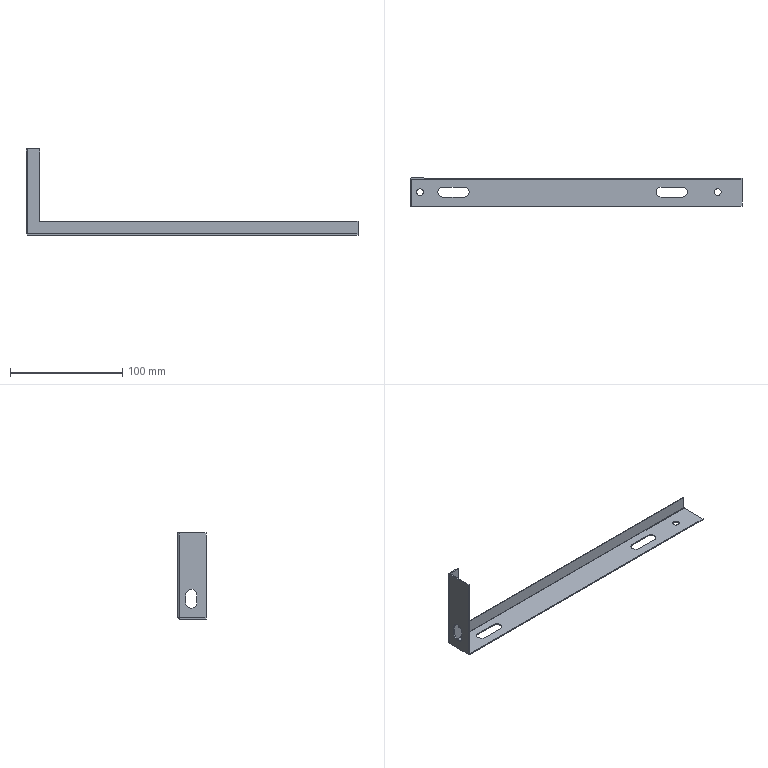Part | SolidWorks | features Cut 2, EdgeFlange 2, FlatPattern 1, ICE 1, LPattern 1, SMBaseFlange 1, SheetMetal 1 | 1 solid | 40 faces | box 296 x 25 x 76.7 mm | volume 12498 mm3 | plane 26 | cylinder 14 | commonest cylinder face diameters 6 x4 9 x4 0.4 x2 2.4 x2 10 x2
STEP:
#1=CARTESIAN_POINT('',(125.7,-15.5,-0.2));
#2=VERTEX_POINT('',#1);
#3=CARTESIAN_POINT('',(125.7,-9.5,-0.2));
#4=VERTEX_POINT('',#3);
#5=CARTESIAN_POINT('',(125.7,-12.5,-0.2));
#6=DIRECTION('',(0.,0.,-1.));
#7=DIRECTION('',(0.,1.,0.));
#8=AXIS2_PLACEMENT_3D('',#5,#6,#7);
#9=CIRCLE('',#8,3.);
#10=EDGE_CURVE('',#2,#4,#9,.T.);
#11=ORIENTED_EDGE('',*,*,#10,.F.);
#12=CARTESIAN_POINT('',(125.7,-15.5,-1.2));
#13=VERTEX_POINT('',#12);
#14=CARTESIAN_POINT('',(125.7,-15.5,8.8));
#15=DIRECTION('',(0.,0.,-1.));
#16=VECTOR('',#15,1000.);
#17=LINE('',#14,#16);
#18=EDGE_CURVE('',#2,#13,#17,.T.);
#19=ORIENTED_EDGE('',*,*,#18,.T.);
#20=CARTESIAN_POINT('',(125.7,-9.5,-1.2));
#21=VERTEX_POINT('',#20);
#22=CARTESIAN_POINT('',(125.7,-12.5,-1.2));
#23=DIRECTION('',(0.,0.,-1.));
#24=DIRECTION('',(0.,1.,0.));
#25=AXIS2_PLACEMENT_3D('',#22,#23,#24);
#26=CIRCLE('',#25,3.);
#27=EDGE_CURVE('',#13,#21,#26,.T.);
#28=ORIENTED_EDGE('',*,*,#27,.T.);
#29=CARTESIAN_POINT('',(125.7,-9.5,8.8));
#30=DIRECTION('',(0.,0.,-1.));
#31=VECTOR('',#30,1000.);
#32=LINE('',#29,#31);
#33=EDGE_CURVE('',#4,#21,#32,.T.);
#34=ORIENTED_EDGE('',*,*,#33,.F.);
#35=EDGE_LOOP('',(#11,#19,#28,#34));
#36=FACE_OUTER_BOUND('',#35,.T.);
#37=CARTESIAN_POINT('',(125.7,-12.5,8.8));
#38=DIRECTION('',(0.,0.,-1.));
#39=DIRECTION('',(0.,1.,0.));
#40=AXIS2_PLACEMENT_3D('',#37,#38,#39);
#41=CYLINDRICAL_SURFACE('',#40,3.);
#42=ADVANCED_FACE('',(#36),#41,.F.);
#43=CARTESIAN_POINT('',(-139.8,-15.5,-0.2));
#44=VERTEX_POINT('',#43);
#45=CARTESIAN_POINT('',(-139.8,-9.5,-0.2));
#46=VERTEX_POINT('',#45);
#47=CARTESIAN_POINT('',(-139.8,-12.5,-0.2));
#48=DIRECTION('',(0.,0.,-1.));
#49=DIRECTION('',(0.,1.,0.));
#50=AXIS2_PLACEMENT_3D('',#47,#48,#49);
#51=CIRCLE('',#50,3.);
#52=EDGE_CURVE('',#44,#46,#51,.T.);
#53=ORIENTED_EDGE('',*,*,#52,.F.);
#54=CARTESIAN_POINT('',(-139.8,-15.5,-1.2));
#55=VERTEX_POINT('',#54);
#56=CARTESIAN_POINT('',(-139.8,-15.5,8.8));
#57=DIRECTION('',(0.,0.,-1.));
#58=VECTOR('',#57,1000.);
#59=LINE('',#56,#58);
#60=EDGE_CURVE('',#44,#55,#59,.T.);
#61=ORIENTED_EDGE('',*,*,#60,.T.);
#62=CARTESIAN_POINT('',(-139.8,-9.5,-1.2));
#63=VERTEX_POINT('',#62);
#64=CARTESIAN_POINT('',(-139.8,-12.5,-1.2));
#65=DIRECTION('',(0.,0.,-1.));
#66=DIRECTION('',(0.,1.,0.));
#67=AXIS2_PLACEMENT_3D('',#64,#65,#66);
#68=CIRCLE('',#67,3.);
#69=EDGE_CURVE('',#55,#63,#68,.T.);
#70=ORIENTED_EDGE('',*,*,#69,.T.);
#71=CARTESIAN_POINT('',(-139.8,-9.5,8.8));
#72=DIRECTION('',(0.,0.,-1.));
#73=VECTOR('',#72,1000.);
#74=LINE('',#71,#73);
#75=EDGE_CURVE('',#46,#63,#74,.T.);
#76=ORIENTED_EDGE('',*,*,#75,.F.);
#77=EDGE_LOOP('',(#53,#61,#70,#76));
#78=FACE_OUTER_BOUND('',#77,.T.);
#79=CARTESIAN_POINT('',(-139.8,-12.5,8.8));
#80=DIRECTION('',(0.,0.,-1.));
#81=DIRECTION('',(0.,1.,0.));
#82=AXIS2_PLACEMENT_3D('',#79,#80,#81);
#83=CYLINDRICAL_SURFACE('',#82,3.);
#84=ADVANCED_FACE('',(#78),#83,.F.);
#85=CARTESIAN_POINT('',(147.4,-1.,11.));
#86=VERTEX_POINT('',#85);
#87=CARTESIAN_POINT('',(-136.4,-1.,11.));
#88=VERTEX_POINT('',#87);
#89=CARTESIAN_POINT('',(-147.4,-1.,11.));
#90=DIRECTION('',(-1.,0.,0.));
#91=VECTOR('',#90,1000.);
#92=LINE('',#89,#91);
#93=EDGE_CURVE('',#86,#88,#92,.T.);
#94=ORIENTED_EDGE('',*,*,#93,.T.);
#95=CARTESIAN_POINT('',(-136.4,-1.,75.5));
#96=VERTEX_POINT('',#95);
#97=CARTESIAN_POINT('',(-136.4,-1.,75.5));
#98=DIRECTION('',(0.,0.,1.));
#99=VECTOR('',#98,1000.);
#100=LINE('',#97,#99);
#101=EDGE_CURVE('',#88,#96,#100,.T.);
#102=ORIENTED_EDGE('',*,*,#101,.T.);
#103=CARTESIAN_POINT('',(-147.4,-1.,75.5));
#104=VERTEX_POINT('',#103);
#105=CARTESIAN_POINT('',(-147.4,-1.,75.5));
#106=DIRECTION('',(1.,0.,0.));
#107=VECTOR('',#106,1000.);
#108=LINE('',#105,#107);
#109=EDGE_CURVE('',#104,#96,#108,.T.);
#110=ORIENTED_EDGE('',*,*,#109,.F.);
#111=CARTESIAN_POINT('',(-147.4,-1.,0.));
#112=VERTEX_POINT('',#111);
#113=CARTESIAN_POINT('',(-147.4,-1.,75.5));
#114=DIRECTION('',(0.,0.,-1.));
#115=VECTOR('',#114,1000.);
#116=LINE('',#113,#115);
#117=EDGE_CURVE('',#104,#112,#116,.T.);
#118=ORIENTED_EDGE('',*,*,#117,.T.);
#119=CARTESIAN_POINT('',(147.4,-1.,0.));
#120=VERTEX_POINT('',#119);
#121=CARTESIAN_POINT('',(-147.4,-1.,0.));
#122=DIRECTION('',(1.,0.,0.));
#123=VECTOR('',#122,1000.);
#124=LINE('',#121,#123);
#125=EDGE_CURVE('',#112,#120,#124,.T.);
#126=ORIENTED_EDGE('',*,*,#125,.T.);
#127=CARTESIAN_POINT('',(147.4,-1.,75.5));
#128=DIRECTION('',(0.,0.,-1.));
#129=VECTOR('',#128,1000.);
#130=LINE('',#127,#129);
#131=EDGE_CURVE('',#86,#120,#130,.T.);
#132=ORIENTED_EDGE('',*,*,#131,.F.);
#133=EDGE_LOOP('',(#94,#102,#110,#118,#126,#132));
#134=FACE_OUTER_BOUND('',#133,.T.);
#135=CARTESIAN_POINT('',(-147.4,-1.,75.5));
#136=DIRECTION('',(0.,1.,0.));
#137=DIRECTION('',(-1.,0.,0.));
#138=AXIS2_PLACEMENT_3D('',#135,#136,#137);
#139=PLANE('',#138);
#140=ADVANCED_FACE('',(#134),#139,.F.);
#141=CARTESIAN_POINT('',(147.4,0.,11.));
#142=VERTEX_POINT('',#141);
#143=CARTESIAN_POINT('',(147.4,-10.,11.));
#144=DIRECTION('',(0.,1.,0.));
#145=VECTOR('',#144,1000.);
#146=LINE('',#143,#145);
#147=EDGE_CURVE('',#86,#142,#146,.T.);
#148=ORIENTED_EDGE('',*,*,#147,.F.);
#149=ORIENTED_EDGE('',*,*,#131,.T.);
#150=CARTESIAN_POINT('',(147.4,0.,0.));
#151=VERTEX_POINT('',#150);
#152=CARTESIAN_POINT('',(147.4,0.,0.));
#153=DIRECTION('',(0.,-1.,0.));
#154=VECTOR('',#153,1000.);
#155=LINE('',#152,#154);
#156=EDGE_CURVE('',#151,#120,#155,.T.);
#157=ORIENTED_EDGE('',*,*,#156,.F.);
#158=CARTESIAN_POINT('',(147.4,0.,75.5));
#159=DIRECTION('',(0.,0.,-1.));
#160=VECTOR('',#159,1000.);
#161=LINE('',#158,#160);
#162=EDGE_CURVE('',#142,#151,#161,.T.);
#163=ORIENTED_EDGE('',*,*,#162,.F.);
#164=EDGE_LOOP('',(#148,#149,#157,#163));
#165=FACE_OUTER_BOUND('',#164,.T.);
#166=CARTESIAN_POINT('',(147.4,0.,75.5));
#167=DIRECTION('',(1.,0.,0.));
#168=DIRECTION('',(0.,0.,-1.));
#169=AXIS2_PLACEMENT_3D('',#166,#167,#168);
#170=PLANE('',#169);
#171=ADVANCED_FACE('',(#165),#170,.T.);
#172=CARTESIAN_POINT('',(-136.4,0.,11.));
#173=VERTEX_POINT('',#172);
#174=CARTESIAN_POINT('',(-136.4,0.,75.5));
#175=VERTEX_POINT('',#174);
#176=CARTESIAN_POINT('',(-136.4,0.,75.5));
#177=DIRECTION('',(0.,0.,1.));
#178=VECTOR('',#177,1000.);
#179=LINE('',#176,#178);
#180=EDGE_CURVE('',#173,#175,#179,.T.);
#181=ORIENTED_EDGE('',*,*,#180,.F.);
#182=CARTESIAN_POINT('',(147.4,0.,11.));
#183=DIRECTION('',(-1.,0.,0.));
#184=VECTOR('',#183,1000.);
#185=LINE('',#182,#184);
#186=EDGE_CURVE('',#142,#173,#185,.T.);
#187=ORIENTED_EDGE('',*,*,#186,.F.);
#188=ORIENTED_EDGE('',*,*,#162,.T.);
#189=CARTESIAN_POINT('',(-147.4,0.,0.));
#190=VERTEX_POINT('',#189);
#191=CARTESIAN_POINT('',(-147.4,0.,0.));
#192=DIRECTION('',(1.,0.,0.));
#193=VECTOR('',#192,1000.);
#194=LINE('',#191,#193);
#195=EDGE_CURVE('',#190,#151,#194,.T.);
#196=ORIENTED_EDGE('',*,*,#195,.F.);
#197=CARTESIAN_POINT('',(-147.4,0.,75.5));
#198=VERTEX_POINT('',#197);
#199=CARTESIAN_POINT('',(-147.4,0.,75.5));
#200=DIRECTION('',(0.,0.,-1.));
#201=VECTOR('',#200,1000.);
#202=LINE('',#199,#201);
#203=EDGE_CURVE('',#198,#190,#202,.T.);
#204=ORIENTED_EDGE('',*,*,#203,.F.);
#205=CARTESIAN_POINT('',(-147.4,0.,75.5));
#206=DIRECTION('',(1.,0.,0.));
#207=VECTOR('',#206,1000.);
#208=LINE('',#205,#207);
#209=EDGE_CURVE('',#198,#175,#208,.T.);
#210=ORIENTED_EDGE('',*,*,#209,.T.);
#211=EDGE_LOOP('',(#181,#187,#188,#196,#204,#210));
#212=FACE_OUTER_BOUND('',#211,.T.);
#213=CARTESIAN_POINT('',(-147.4,0.,75.5));
#214=DIRECTION('',(0.,1.,0.));
#215=DIRECTION('',(-1.,0.,0.));
#216=AXIS2_PLACEMENT_3D('',#213,#214,#215);
#217=PLANE('',#216);
#218=ADVANCED_FACE('',(#212),#217,.T.);
#219=ORIENTED_EDGE('',*,*,#109,.T.);
#220=CARTESIAN_POINT('',(-136.4,0.,75.5));
#221=DIRECTION('',(0.,1.,0.));
#222=VECTOR('',#221,1000.);
#223=LINE('',#220,#222);
#224=EDGE_CURVE('',#96,#175,#223,.T.);
#225=ORIENTED_EDGE('',*,*,#224,.T.);
#226=ORIENTED_EDGE('',*,*,#209,.F.);
#227=CARTESIAN_POINT('',(-147.4,-1.,75.5));
#228=DIRECTION('',(0.,1.,0.));
#229=VECTOR('',#228,1000.);
#230=LINE('',#227,#229);
#231=EDGE_CURVE('',#104,#198,#230,.T.);
#232=ORIENTED_EDGE('',*,*,#231,.F.);
#233=EDGE_LOOP('',(#219,#225,#226,#232));
#234=FACE_OUTER_BOUND('',#233,.T.);
#235=CARTESIAN_POINT('',(0.,0.,75.5));
#236=DIRECTION('',(0.,0.,-1.));
#237=DIRECTION('',(-1.,0.,0.));
#238=AXIS2_PLACEMENT_3D('',#235,#236,#237);
#239=PLANE('',#238);
#240=ADVANCED_FACE('',(#234),#239,.F.);
#241=ORIENTED_EDGE('',*,*,#147,.T.);
#242=ORIENTED_EDGE('',*,*,#186,.T.);
#243=CARTESIAN_POINT('',(-136.4,-10.,11.));
#244=DIRECTION('',(0.,1.,0.));
#245=VECTOR('',#244,1000.);
#246=LINE('',#243,#245);
#247=EDGE_CURVE('',#88,#173,#246,.T.);
#248=ORIENTED_EDGE('',*,*,#247,.F.);
#249=ORIENTED_EDGE('',*,*,#93,.F.);
#250=EDGE_LOOP('',(#241,#242,#248,#249));
#251=FACE_OUTER_BOUND('',#250,.T.);
#252=CARTESIAN_POINT('',(147.4,-10.,11.));
#253=DIRECTION('',(0.,0.,-1.));
#254=DIRECTION('',(-1.,0.,0.));
#255=AXIS2_PLACEMENT_3D('',#252,#253,#254);
#256=PLANE('',#255);
#257=ADVANCED_FACE('',(#251),#256,.F.);
#258=ORIENTED_EDGE('',*,*,#247,.T.);
#259=ORIENTED_EDGE('',*,*,#180,.T.);
#260=ORIENTED_EDGE('',*,*,#224,.F.);
#261=ORIENTED_EDGE('',*,*,#101,.F.);
#262=EDGE_LOOP('',(#258,#259,#260,#261));
#263=FACE_OUTER_BOUND('',#262,.T.);
#264=CARTESIAN_POINT('',(-136.4,-10.,75.5));
#265=DIRECTION('',(-1.,0.,0.));
#266=DIRECTION('',(0.,0.,1.));
#267=AXIS2_PLACEMENT_3D('',#264,#265,#266);
#268=PLANE('',#267);
#269=ADVANCED_FACE('',(#263),#268,.F.);
#270=CARTESIAN_POINT('',(-147.4,-1.2,-0.2));
#271=VERTEX_POINT('',#270);
#272=CARTESIAN_POINT('',(-147.4,-1.2,-1.2));
#273=VERTEX_POINT('',#272);
#274=CARTESIAN_POINT('',(-147.4,-1.2,-1.2));
#275=DIRECTION('',(0.,0.,-1.));
#276=VECTOR('',#275,1000.);
#277=LINE('',#274,#276);
#278=EDGE_CURVE('',#271,#273,#277,.T.);
#279=ORIENTED_EDGE('',*,*,#278,.F.);
#280=CARTESIAN_POINT('',(-147.4,-1.2,0.));
#281=DIRECTION('',(-1.,0.,0.));
#282=DIRECTION('',(0.,1.,0.));
#283=AXIS2_PLACEMENT_3D('',#280,#281,#282);
#284=CIRCLE('',#283,0.2);
#285=EDGE_CURVE('',#112,#271,#284,.T.);
#286=ORIENTED_EDGE('',*,*,#285,.F.);
#287=CARTESIAN_POINT('',(-147.4,-1.,0.));
#288=DIRECTION('',(0.,1.,0.));
#289=VECTOR('',#288,1000.);
#290=LINE('',#287,#289);
#291=EDGE_CURVE('',#112,#190,#290,.T.);
#292=ORIENTED_EDGE('',*,*,#291,.T.);
#293=CARTESIAN_POINT('',(-147.4,-1.2,0.));
#294=DIRECTION('',(-1.,0.,0.));
#295=DIRECTION('',(0.,1.,0.));
#296=AXIS2_PLACEMENT_3D('',#293,#294,#295);
#297=CIRCLE('',#296,1.2);
#298=EDGE_CURVE('',#190,#273,#297,.T.);
#299=ORIENTED_EDGE('',*,*,#298,.T.);
#300=EDGE_LOOP('',(#279,#286,#292,#299));
#301=FACE_OUTER_BOUND('',#300,.T.);
#302=CARTESIAN_POINT('',(-147.4,-1.2,0.));
#303=DIRECTION('',(-1.,0.,0.));
#304=DIRECTION('',(0.,-1.,0.));
#305=AXIS2_PLACEMENT_3D('',#302,#303,#304);
#306=PLANE('',#305);
#307=ADVANCED_FACE('',(#301),#306,.T.);
#308=CARTESIAN_POINT('',(147.4,-1.2,-0.2));
#309=VERTEX_POINT('',#308);
#310=CARTESIAN_POINT('',(147.4,-1.2,0.));
#311=DIRECTION('',(1.,0.,0.));
#312=DIRECTION('',(0.,1.,0.));
#313=AXIS2_PLACEMENT_3D('',#310,#311,#312);
#314=CIRCLE('',#313,0.2);
#315=EDGE_CURVE('',#309,#120,#314,.T.);
#316=ORIENTED_EDGE('',*,*,#315,.F.);
#317=CARTESIAN_POINT('',(147.4,-1.2,-1.2));
#318=VERTEX_POINT('',#317);
#319=CARTESIAN_POINT('',(147.4,-1.2,-0.2));
#320=DIRECTION('',(0.,0.,-1.));
#321=VECTOR('',#320,1000.);
#322=LINE('',#319,#321);
#323=EDGE_CURVE('',#309,#318,#322,.T.);
#324=ORIENTED_EDGE('',*,*,#323,.T.);
#325=CARTESIAN_POINT('',(147.4,-1.2,0.));
#326=DIRECTION('',(1.,0.,0.));
#327=DIRECTION('',(0.,1.,0.));
#328=AXIS2_PLACEMENT_3D('',#325,#326,#327);
#329=CIRCLE('',#328,1.2);
#330=EDGE_CURVE('',#318,#151,#329,.T.);
#331=ORIENTED_EDGE('',*,*,#330,.T.);
#332=ORIENTED_EDGE('',*,*,#156,.T.);
#333=EDGE_LOOP('',(#316,#324,#331,#332));
#334=FACE_OUTER_BOUND('',#333,.T.);
#335=CARTESIAN_POINT('',(147.4,-1.2,0.));
#336=DIRECTION('',(-1.,0.,0.));
#337=DIRECTION('',(0.,-1.,0.));
#338=AXIS2_PLACEMENT_3D('',#335,#336,#337);
#339=PLANE('',#338);
#340=ADVANCED_FACE('',(#334),#339,.F.);
#341=ORIENTED_EDGE('',*,*,#195,.T.);
#342=ORIENTED_EDGE('',*,*,#330,.F.);
#343=CARTESIAN_POINT('',(0.,-1.2,-1.2));
#344=DIRECTION('',(1.,0.,0.));
#345=VECTOR('',#344,1000.);
#346=LINE('',#343,#345);
#347=EDGE_CURVE('',#273,#318,#346,.T.);
#348=ORIENTED_EDGE('',*,*,#347,.F.);
#349=ORIENTED_EDGE('',*,*,#298,.F.);
#350=EDGE_LOOP('',(#341,#342,#348,#349));
#351=FACE_OUTER_BOUND('',#350,.T.);
#352=CARTESIAN_POINT('',(147.4,-1.2,0.));
#353=DIRECTION('',(1.,0.,0.));
#354=DIRECTION('',(0.,0.,-1.));
#355=AXIS2_PLACEMENT_3D('',#352,#353,#354);
#356=CYLINDRICAL_SURFACE('',#355,1.2);
#357=ADVANCED_FACE('',(#351),#356,.T.);
#358=ORIENTED_EDGE('',*,*,#125,.F.);
#359=ORIENTED_EDGE('',*,*,#285,.T.);
#360=CARTESIAN_POINT('',(-147.4,-1.2,-0.2));
#361=DIRECTION('',(1.,0.,0.));
#362=VECTOR('',#361,1000.);
#363=LINE('',#360,#362);
#364=EDGE_CURVE('',#271,#309,#363,.T.);
#365=ORIENTED_EDGE('',*,*,#364,.T.);
#366=ORIENTED_EDGE('',*,*,#315,.T.);
#367=EDGE_LOOP('',(#358,#359,#365,#366));
#368=FACE_OUTER_BOUND('',#367,.T.);
#369=CARTESIAN_POINT('',(147.4,-1.2,0.));
#370=DIRECTION('',(1.,0.,0.));
#371=DIRECTION('',(0.,0.,-1.));
#372=AXIS2_PLACEMENT_3D('',#369,#370,#371);
#373=CYLINDRICAL_SURFACE('',#372,0.2);
#374=ADVANCED_FACE('',(#368),#373,.F.);
#375=CARTESIAN_POINT('',(147.4,-25.,-1.2));
#376=VERTEX_POINT('',#375);
#377=CARTESIAN_POINT('',(147.4,-1.,-1.2));
#378=DIRECTION('',(0.,1.,0.));
#379=VECTOR('',#378,1000.);
#380=LINE('',#377,#379);
#381=EDGE_CURVE('',#376,#318,#380,.T.);
#382=ORIENTED_EDGE('',*,*,#381,.T.);
#383=ORIENTED_EDGE('',*,*,#323,.F.);
#384=CARTESIAN_POINT('',(147.4,-25.,-0.2));
#385=VERTEX_POINT('',#384);
#386=CARTESIAN_POINT('',(147.4,0.,-0.2));
#387=DIRECTION('',(0.,1.,0.));
#388=VECTOR('',#387,1000.);
#389=LINE('',#386,#388);
#390=EDGE_CURVE('',#385,#309,#389,.T.);
#391=ORIENTED_EDGE('',*,*,#390,.F.);
#392=CARTESIAN_POINT('',(147.4,-25.,-1.2));
#393=DIRECTION('',(0.,0.,1.));
#394=VECTOR('',#393,1000.);
#395=LINE('',#392,#394);
#396=EDGE_CURVE('',#376,#385,#395,.T.);
#397=ORIENTED_EDGE('',*,*,#396,.F.);
#398=EDGE_LOOP('',(#382,#383,#391,#397));
#399=FACE_OUTER_BOUND('',#398,.T.);
#400=CARTESIAN_POINT('',(147.4,-1.,-1.2));
#401=DIRECTION('',(1.,0.,0.));
#402=DIRECTION('',(0.,0.,-1.));
#403=AXIS2_PLACEMENT_3D('',#400,#401,#402);
#404=PLANE('',#403);
#405=ADVANCED_FACE('',(#399),#404,.T.);
#406=CARTESIAN_POINT('',(-147.4,-25.,-0.2));
#407=VERTEX_POINT('',#406);
#408=CARTESIAN_POINT('',(-147.4,0.,-0.2));
#409=DIRECTION('',(0.,-1.,0.));
#410=VECTOR('',#409,1000.);
#411=LINE('',#408,#410);
#412=EDGE_CURVE('',#271,#407,#411,.T.);
#413=ORIENTED_EDGE('',*,*,#412,.F.);
#414=ORIENTED_EDGE('',*,*,#278,.T.);
#415=CARTESIAN_POINT('',(-147.4,-25.,-1.2));
#416=VERTEX_POINT('',#415);
#417=CARTESIAN_POINT('',(-147.4,-25.,-1.2));
#418=DIRECTION('',(0.,-1.,0.));
#419=VECTOR('',#418,1000.);
#420=LINE('',#417,#419);
#421=EDGE_CURVE('',#273,#416,#420,.T.);
#422=ORIENTED_EDGE('',*,*,#421,.T.);
#423=CARTESIAN_POINT('',(-147.4,-25.,-1.2));
#424=DIRECTION('',(0.,0.,1.));
#425=VECTOR('',#424,1000.);
#426=LINE('',#423,#425);
#427=EDGE_CURVE('',#416,#407,#426,.T.);
#428=ORIENTED_EDGE('',*,*,#427,.T.);
#429=EDGE_LOOP('',(#413,#414,#422,#428));
#430=FACE_OUTER_BOUND('',#429,.T.);
#431=CARTESIAN_POINT('',(-147.4,-25.,-1.2));
#432=DIRECTION('',(-1.,0.,0.));
#433=DIRECTION('',(0.,0.,1.));
#434=AXIS2_PLACEMENT_3D('',#431,#432,#433);
#435=PLANE('',#434);
#436=ADVANCED_FACE('',(#430),#435,.T.);
#437=CARTESIAN_POINT('',(125.7,-12.5,-1.2));
#438=DIRECTION('',(0.,0.,-1.));
#439=DIRECTION('',(0.,1.,0.));
#440=AXIS2_PLACEMENT_3D('',#437,#438,#439);
#441=CIRCLE('',#440,3.);
#442=EDGE_CURVE('',#21,#13,#441,.T.);
#443=ORIENTED_EDGE('',*,*,#442,.F.);
#444=ORIENTED_EDGE('',*,*,#27,.F.);
#445=EDGE_LOOP('',(#443,#444));
#446=FACE_BOUND('',#445,.T.);
#447=CARTESIAN_POINT('',(-139.8,-12.5,-1.2));
#448=DIRECTION('',(0.,0.,-1.));
#449=DIRECTION('',(0.,1.,0.));
#450=AXIS2_PLACEMENT_3D('',#447,#448,#449);
#451=CIRCLE('',#450,3.);
#452=EDGE_CURVE('',#63,#55,#451,.T.);
#453=ORIENTED_EDGE('',*,*,#452,.F.);
#454=ORIENTED_EDGE('',*,*,#69,.F.);
#455=EDGE_LOOP('',(#453,#454));
#456=FACE_BOUND('',#455,.T.);
#457=CARTESIAN_POINT('',(75.2,-17.,-1.2));
#458=VERTEX_POINT('',#457);
#459=CARTESIAN_POINT('',(75.2,-8.,-1.2));
#460=VERTEX_POINT('',#459);
#461=CARTESIAN_POINT('',(75.2,-12.5,-1.2));
#462=DIRECTION('',(0.,0.,-1.));
#463=DIRECTION('',(0.,1.,0.));
#464=AXIS2_PLACEMENT_3D('',#461,#462,#463);
#465=CIRCLE('',#464,4.5);
#466=EDGE_CURVE('',#458,#460,#465,.T.);
#467=ORIENTED_EDGE('',*,*,#466,.F.);
#468=CARTESIAN_POINT('',(94.2,-17.,-1.2));
#469=VERTEX_POINT('',#468);
#470=CARTESIAN_POINT('',(75.2,-17.,-1.2));
#471=DIRECTION('',(-1.,0.,0.));
#472=VECTOR('',#471,1000.);
#473=LINE('',#470,#472);
#474=EDGE_CURVE('',#469,#458,#473,.T.);
#475=ORIENTED_EDGE('',*,*,#474,.F.);
#476=CARTESIAN_POINT('',(94.2,-8.,-1.2));
#477=VERTEX_POINT('',#476);
#478=CARTESIAN_POINT('',(94.2,-12.5,-1.2));
#479=DIRECTION('',(0.,0.,-1.));
#480=DIRECTION('',(0.,1.,0.));
#481=AXIS2_PLACEMENT_3D('',#478,#479,#480);
#482=CIRCLE('',#481,4.5);
#483=EDGE_CURVE('',#477,#469,#482,.T.);
#484=ORIENTED_EDGE('',*,*,#483,.F.);
#485=CARTESIAN_POINT('',(75.2,-8.,-1.2));
#486=DIRECTION('',(1.,0.,0.));
#487=VECTOR('',#486,1000.);
#488=LINE('',#485,#487);
#489=EDGE_CURVE('',#460,#477,#488,.T.);
#490=ORIENTED_EDGE('',*,*,#489,.F.);
#491=EDGE_LOOP('',(#467,#475,#484,#490));
#492=FACE_BOUND('',#491,.T.);
#493=CARTESIAN_POINT('',(-119.3,-17.,-1.2));
#494=VERTEX_POINT('',#493);
#495=CARTESIAN_POINT('',(-119.3,-8.,-1.2));
#496=VERTEX_POINT('',#495);
#497=CARTESIAN_POINT('',(-119.3,-12.5,-1.2));
#498=DIRECTION('',(0.,0.,-1.));
#499=DIRECTION('',(0.,1.,0.));
#500=AXIS2_PLACEMENT_3D('',#497,#498,#499);
#501=CIRCLE('',#500,4.5);
#502=EDGE_CURVE('',#494,#496,#501,.T.);
#503=ORIENTED_EDGE('',*,*,#502,.F.);
#504=CARTESIAN_POINT('',(-100.3,-17.,-1.2));
#505=VERTEX_POINT('',#504);
#506=CARTESIAN_POINT('',(-119.3,-17.,-1.2));
#507=DIRECTION('',(-1.,0.,0.));
#508=VECTOR('',#507,1000.);
#509=LINE('',#506,#508);
#510=EDGE_CURVE('',#505,#494,#509,.T.);
#511=ORIENTED_EDGE('',*,*,#510,.F.);
#512=CARTESIAN_POINT('',(-100.3,-8.,-1.2));
#513=VERTEX_POINT('',#512);
#514=CARTESIAN_POINT('',(-100.3,-12.5,-1.2));
#515=DIRECTION('',(0.,0.,-1.));
#516=DIRECTION('',(0.,1.,0.));
#517=AXIS2_PLACEMENT_3D('',#514,#515,#516);
#518=CIRCLE('',#517,4.5);
#519=EDGE_CURVE('',#513,#505,#518,.T.);
#520=ORIENTED_EDGE('',*,*,#519,.F.);
#521=CARTESIAN_POINT('',(-119.3,-8.,-1.2));
#522=DIRECTION('',(1.,0.,0.));
#523=VECTOR('',#522,1000.);
#524=LINE('',#521,#523);
#525=EDGE_CURVE('',#496,#513,#524,.T.);
#526=ORIENTED_EDGE('',*,*,#525,.F.);
#527=EDGE_LOOP('',(#503,#511,#520,#526));
#528=FACE_BOUND('',#527,.T.);
#529=ORIENTED_EDGE('',*,*,#421,.F.);
#530=ORIENTED_EDGE('',*,*,#347,.T.);
#531=ORIENTED_EDGE('',*,*,#381,.F.);
#532=CARTESIAN_POINT('',(147.4,-25.,-1.2));
#533=DIRECTION('',(1.,0.,0.));
#534=VECTOR('',#533,1000.);
#535=LINE('',#532,#534);
#536=EDGE_CURVE('',#416,#376,#535,.T.);
#537=ORIENTED_EDGE('',*,*,#536,.F.);
#538=EDGE_LOOP('',(#529,#530,#531,#537));
#539=FACE_OUTER_BOUND('',#538,.T.);
#540=CARTESIAN_POINT('',(0.,0.,-1.2));
#541=DIRECTION('',(0.,0.,-1.));
#542=DIRECTION('',(0.,1.,0.));
#543=AXIS2_PLACEMENT_3D('',#540,#541,#542);
#544=PLANE('',#543);
#545=ADVANCED_FACE('',(#446,#456,#492,#528,#539),#544,.T.);
#546=CARTESIAN_POINT('',(125.7,-12.5,-0.2));
#547=DIRECTION('',(0.,0.,-1.));
#548=DIRECTION('',(0.,1.,0.));
#549=AXIS2_PLACEMENT_3D('',#546,#547,#548);
#550=CIRCLE('',#549,3.);
#551=EDGE_CURVE('',#4,#2,#550,.T.);
#552=ORIENTED_EDGE('',*,*,#551,.T.);
#553=ORIENTED_EDGE('',*,*,#10,.T.);
#554=EDGE_LOOP('',(#552,#553));
#555=FACE_BOUND('',#554,.T.);
#556=CARTESIAN_POINT('',(-139.8,-12.5,-0.2));
#557=DIRECTION('',(0.,0.,-1.));
#558=DIRECTION('',(0.,1.,0.));
#559=AXIS2_PLACEMENT_3D('',#556,#557,#558);
#560=CIRCLE('',#559,3.);
#561=EDGE_CURVE('',#46,#44,#560,.T.);
#562=ORIENTED_EDGE('',*,*,#561,.T.);
#563=ORIENTED_EDGE('',*,*,#52,.T.);
#564=EDGE_LOOP('',(#562,#563));
#565=FACE_BOUND('',#564,.T.);
#566=CARTESIAN_POINT('',(94.2,-17.,-0.2));
#567=VERTEX_POINT('',#566);
#568=CARTESIAN_POINT('',(75.2,-17.,-0.2));
#569=VERTEX_POINT('',#568);
#570=CARTESIAN_POINT('',(0.,-17.,-0.2));
#571=DIRECTION('',(-1.,0.,0.));
#572=VECTOR('',#571,1000.);
#573=LINE('',#570,#572);
#574=EDGE_CURVE('',#567,#569,#573,.T.);
#575=ORIENTED_EDGE('',*,*,#574,.T.);
#576=CARTESIAN_POINT('',(75.2,-8.,-0.2));
#577=VERTEX_POINT('',#576);
#578=CARTESIAN_POINT('',(75.2,-12.5,-0.2));
#579=DIRECTION('',(0.,0.,-1.));
#580=DIRECTION('',(0.,1.,0.));
#581=AXIS2_PLACEMENT_3D('',#578,#579,#580);
#582=CIRCLE('',#581,4.5);
#583=EDGE_CURVE('',#569,#577,#582,.T.);
#584=ORIENTED_EDGE('',*,*,#583,.T.);
#585=CARTESIAN_POINT('',(94.2,-8.,-0.2));
#586=VERTEX_POINT('',#585);
#587=CARTESIAN_POINT('',(0.,-8.,-0.2));
#588=DIRECTION('',(1.,0.,0.));
#589=VECTOR('',#588,1000.);
#590=LINE('',#587,#589);
#591=EDGE_CURVE('',#577,#586,#590,.T.);
#592=ORIENTED_EDGE('',*,*,#591,.T.);
#593=CARTESIAN_POINT('',(94.2,-12.5,-0.2));
#594=DIRECTION('',(0.,0.,-1.));
#595=DIRECTION('',(0.,1.,0.));
#596=AXIS2_PLACEMENT_3D('',#593,#594,#595);
#597=CIRCLE('',#596,4.5);
#598=EDGE_CURVE('',#586,#567,#597,.T.);
#599=ORIENTED_EDGE('',*,*,#598,.T.);
#600=EDGE_LOOP('',(#575,#584,#592,#599));
#601=FACE_BOUND('',#600,.T.);
#602=CARTESIAN_POINT('',(-100.3,-17.,-0.2));
#603=VERTEX_POINT('',#602);
#604=CARTESIAN_POINT('',(-119.3,-17.,-0.2));
#605=VERTEX_POINT('',#604);
#606=CARTESIAN_POINT('',(0.,-17.,-0.2));
#607=DIRECTION('',(-1.,0.,0.));
#608=VECTOR('',#607,1000.);
#609=LINE('',#606,#608);
#610=EDGE_CURVE('',#603,#605,#609,.T.);
#611=ORIENTED_EDGE('',*,*,#610,.T.);
#612=CARTESIAN_POINT('',(-119.3,-8.,-0.2));
#613=VERTEX_POINT('',#612);
#614=CARTESIAN_POINT('',(-119.3,-12.5,-0.2));
#615=DIRECTION('',(0.,0.,-1.));
#616=DIRECTION('',(0.,1.,0.));
#617=AXIS2_PLACEMENT_3D('',#614,#615,#616);
#618=CIRCLE('',#617,4.5);
#619=EDGE_CURVE('',#605,#613,#618,.T.);
#620=ORIENTED_EDGE('',*,*,#619,.T.);
#621=CARTESIAN_POINT('',(-100.3,-8.,-0.2));
#622=VERTEX_POINT('',#621);
#623=CARTESIAN_POINT('',(0.,-8.,-0.2));
#624=DIRECTION('',(1.,0.,0.));
#625=VECTOR('',#624,1000.);
#626=LINE('',#623,#625);
#627=EDGE_CURVE('',#613,#622,#626,.T.);
#628=ORIENTED_EDGE('',*,*,#627,.T.);
#629=CARTESIAN_POINT('',(-100.3,-12.5,-0.2));
#630=DIRECTION('',(0.,0.,-1.));
#631=DIRECTION('',(0.,1.,0.));
#632=AXIS2_PLACEMENT_3D('',#629,#630,#631);
#633=CIRCLE('',#632,4.5);
#634=EDGE_CURVE('',#622,#603,#633,.T.);
#635=ORIENTED_EDGE('',*,*,#634,.T.);
#636=EDGE_LOOP('',(#611,#620,#628,#635));
#637=FACE_BOUND('',#636,.T.);
#638=ORIENTED_EDGE('',*,*,#364,.F.);
#639=ORIENTED_EDGE('',*,*,#412,.T.);
#640=CARTESIAN_POINT('',(0.,-25.,-0.2));
#641=DIRECTION('',(1.,0.,0.));
#642=VECTOR('',#641,1000.);
#643=LINE('',#640,#642);
#644=EDGE_CURVE('',#407,#385,#643,.T.);
#645=ORIENTED_EDGE('',*,*,#644,.T.);
#646=ORIENTED_EDGE('',*,*,#390,.T.);
#647=EDGE_LOOP('',(#638,#639,#645,#646));
#648=FACE_OUTER_BOUND('',#647,.T.);
#649=CARTESIAN_POINT('',(0.,0.,-0.2));
#650=DIRECTION('',(0.,0.,-1.));
#651=DIRECTION('',(0.,1.,0.));
#652=AXIS2_PLACEMENT_3D('',#649,#650,#651);
#653=PLANE('',#652);
#654=ADVANCED_FACE('',(#555,#565,#601,#637,#648),#653,.F.);
#655=ORIENTED_EDGE('',*,*,#644,.F.);
#656=ORIENTED_EDGE('',*,*,#427,.F.);
#657=ORIENTED_EDGE('',*,*,#536,.T.);
#658=ORIENTED_EDGE('',*,*,#396,.T.);
#659=EDGE_LOOP('',(#655,#656,#657,#658));
#660=FACE_OUTER_BOUND('',#659,.T.);
#661=CARTESIAN_POINT('',(147.4,-25.,-1.2));
#662=DIRECTION('',(0.,-1.,0.));
#663=DIRECTION('',(0.,0.,-1.));
#664=AXIS2_PLACEMENT_3D('',#661,#662,#663);
#665=PLANE('',#664);
#666=ADVANCED_FACE('',(#660),#665,.T.);
#667=CARTESIAN_POINT('',(-147.6,-1.2,75.5));
#668=VERTEX_POINT('',#667);
#669=CARTESIAN_POINT('',(-148.6,-1.2,75.5));
#670=VERTEX_POINT('',#669);
#671=CARTESIAN_POINT('',(-148.6,-1.2,75.5));
#672=DIRECTION('',(-1.,0.,0.));
#673=VECTOR('',#672,1000.);
#674=LINE('',#671,#673);
#675=EDGE_CURVE('',#668,#670,#674,.T.);
#676=ORIENTED_EDGE('',*,*,#675,.F.);
#677=CARTESIAN_POINT('',(-147.4,-1.2,75.5));
#678=DIRECTION('',(0.,0.,1.));
#679=DIRECTION('',(-1.,0.,0.));
#680=AXIS2_PLACEMENT_3D('',#677,#678,#679);
#681=CIRCLE('',#680,0.2);
#682=EDGE_CURVE('',#104,#668,#681,.T.);
#683=ORIENTED_EDGE('',*,*,#682,.F.);
#684=ORIENTED_EDGE('',*,*,#231,.T.);
#685=CARTESIAN_POINT('',(-147.4,-1.2,75.5));
#686=DIRECTION('',(0.,0.,1.));
#687=DIRECTION('',(-1.,0.,0.));
#688=AXIS2_PLACEMENT_3D('',#685,#686,#687);
#689=CIRCLE('',#688,1.2);
#690=EDGE_CURVE('',#198,#670,#689,.T.);
#691=ORIENTED_EDGE('',*,*,#690,.T.);
#692=EDGE_LOOP('',(#676,#683,#684,#691));
#693=FACE_OUTER_BOUND('',#692,.T.);
#694=CARTESIAN_POINT('',(-147.4,-1.2,75.5));
#695=DIRECTION('',(0.,0.,1.));
#696=DIRECTION('',(1.,0.,0.));
#697=AXIS2_PLACEMENT_3D('',#694,#695,#696);
#698=PLANE('',#697);
#699=ADVANCED_FACE('',(#693),#698,.T.);
#700=CARTESIAN_POINT('',(-147.6,-1.2,0.));
#701=VERTEX_POINT('',#700);
#702=CARTESIAN_POINT('',(-147.4,-1.2,0.));
#703=DIRECTION('',(0.,0.,-1.));
#704=DIRECTION('',(-1.,0.,0.));
#705=AXIS2_PLACEMENT_3D('',#702,#703,#704);
#706=CIRCLE('',#705,0.2);
#707=EDGE_CURVE('',#701,#112,#706,.T.);
#708=ORIENTED_EDGE('',*,*,#707,.F.);
#709=CARTESIAN_POINT('',(-148.6,-1.2,0.));
#710=VERTEX_POINT('',#709);
#711=CARTESIAN_POINT('',(-147.6,-1.2,0.));
#712=DIRECTION('',(-1.,0.,0.));
#713=VECTOR('',#712,1000.);
#714=LINE('',#711,#713);
#715=EDGE_CURVE('',#701,#710,#714,.T.);
#716=ORIENTED_EDGE('',*,*,#715,.T.);
#717=CARTESIAN_POINT('',(-147.4,-1.2,0.));
#718=DIRECTION('',(0.,0.,-1.));
#719=DIRECTION('',(-1.,0.,0.));
#720=AXIS2_PLACEMENT_3D('',#717,#718,#719);
#721=CIRCLE('',#720,1.2);
#722=EDGE_CURVE('',#710,#190,#721,.T.);
#723=ORIENTED_EDGE('',*,*,#722,.T.);
#724=ORIENTED_EDGE('',*,*,#291,.F.);
#725=EDGE_LOOP('',(#708,#716,#723,#724));
#726=FACE_OUTER_BOUND('',#725,.T.);
#727=CARTESIAN_POINT('',(-147.4,-1.2,0.));
#728=DIRECTION('',(0.,0.,1.));
#729=DIRECTION('',(1.,0.,0.));
#730=AXIS2_PLACEMENT_3D('',#727,#728,#729);
#731=PLANE('',#730);
#732=ADVANCED_FACE('',(#726),#731,.F.);
#733=ORIENTED_EDGE('',*,*,#203,.T.);
#734=ORIENTED_EDGE('',*,*,#722,.F.);
#735=CARTESIAN_POINT('',(-148.6,-1.2,0.));
#736=DIRECTION('',(0.,0.,-1.));
#737=VECTOR('',#736,1000.);
#738=LINE('',#735,#737);
#739=EDGE_CURVE('',#670,#710,#738,.T.);
#740=ORIENTED_EDGE('',*,*,#739,.F.);
#741=ORIENTED_EDGE('',*,*,#690,.F.);
#742=EDGE_LOOP('',(#733,#734,#740,#741));
#743=FACE_OUTER_BOUND('',#742,.T.);
#744=CARTESIAN_POINT('',(-147.4,-1.2,0.));
#745=DIRECTION('',(0.,0.,-1.));
#746=DIRECTION('',(-1.,0.,0.));
#747=AXIS2_PLACEMENT_3D('',#744,#745,#746);
#748=CYLINDRICAL_SURFACE('',#747,1.2);
#749=ADVANCED_FACE('',(#743),#748,.T.);
#750=ORIENTED_EDGE('',*,*,#117,.F.);
#751=ORIENTED_EDGE('',*,*,#682,.T.);
#752=CARTESIAN_POINT('',(-147.6,-1.2,75.5));
#753=DIRECTION('',(0.,0.,-1.));
#754=VECTOR('',#753,1000.);
#755=LINE('',#752,#754);
#756=EDGE_CURVE('',#668,#701,#755,.T.);
#757=ORIENTED_EDGE('',*,*,#756,.T.);
#758=ORIENTED_EDGE('',*,*,#707,.T.);
#759=EDGE_LOOP('',(#750,#751,#757,#758));
#760=FACE_OUTER_BOUND('',#759,.T.);
#761=CARTESIAN_POINT('',(-147.4,-1.2,0.));
#762=DIRECTION('',(0.,0.,-1.));
#763=DIRECTION('',(-1.,0.,0.));
#764=AXIS2_PLACEMENT_3D('',#761,#762,#763);
#765=CYLINDRICAL_SURFACE('',#764,0.2);
#766=ADVANCED_FACE('',(#760),#765,.F.);
#767=CARTESIAN_POINT('',(-148.6,-25.,0.));
#768=VERTEX_POINT('',#767);
#769=CARTESIAN_POINT('',(-148.6,-1.,0.));
#770=DIRECTION('',(0.,1.,0.));
#771=VECTOR('',#770,1000.);
#772=LINE('',#769,#771);
#773=EDGE_CURVE('',#768,#710,#772,.T.);
#774=ORIENTED_EDGE('',*,*,#773,.T.);
#775=ORIENTED_EDGE('',*,*,#715,.F.);
#776=CARTESIAN_POINT('',(-147.6,-25.,0.));
#777=VERTEX_POINT('',#776);
#778=CARTESIAN_POINT('',(-147.6,0.,0.));
#779=DIRECTION('',(0.,1.,0.));
#780=VECTOR('',#779,1000.);
#781=LINE('',#778,#780);
#782=EDGE_CURVE('',#777,#701,#781,.T.);
#783=ORIENTED_EDGE('',*,*,#782,.F.);
#784=CARTESIAN_POINT('',(-148.6,-25.,0.));
#785=DIRECTION('',(1.,0.,0.));
#786=VECTOR('',#785,1000.);
#787=LINE('',#784,#786);
#788=EDGE_CURVE('',#768,#777,#787,.T.);
#789=ORIENTED_EDGE('',*,*,#788,.F.);
#790=EDGE_LOOP('',(#774,#775,#783,#789));
#791=FACE_OUTER_BOUND('',#790,.T.);
#792=CARTESIAN_POINT('',(-148.6,-1.,0.));
#793=DIRECTION('',(0.,0.,-1.));
#794=DIRECTION('',(-1.,0.,0.));
#795=AXIS2_PLACEMENT_3D('',#792,#793,#794);
#796=PLANE('',#795);
#797=ADVANCED_FACE('',(#791),#796,.T.);
#798=CARTESIAN_POINT('',(-147.6,-25.,75.5));
#799=VERTEX_POINT('',#798);
#800=CARTESIAN_POINT('',(-147.6,0.,75.5));
#801=DIRECTION('',(0.,-1.,0.));
#802=VECTOR('',#801,1000.);
#803=LINE('',#800,#802);
#804=EDGE_CURVE('',#668,#799,#803,.T.);
#805=ORIENTED_EDGE('',*,*,#804,.F.);
#806=ORIENTED_EDGE('',*,*,#675,.T.);
#807=CARTESIAN_POINT('',(-148.6,-25.,75.5));
#808=VERTEX_POINT('',#807);
#809=CARTESIAN_POINT('',(-148.6,-25.,75.5));
#810=DIRECTION('',(0.,-1.,0.));
#811=VECTOR('',#810,1000.);
#812=LINE('',#809,#811);
#813=EDGE_CURVE('',#670,#808,#812,.T.);
#814=ORIENTED_EDGE('',*,*,#813,.T.);
#815=CARTESIAN_POINT('',(-148.6,-25.,75.5));
#816=DIRECTION('',(1.,0.,0.));
#817=VECTOR('',#816,1000.);
#818=LINE('',#815,#817);
#819=EDGE_CURVE('',#808,#799,#818,.T.);
#820=ORIENTED_EDGE('',*,*,#819,.T.);
#821=EDGE_LOOP('',(#805,#806,#814,#820));
#822=FACE_OUTER_BOUND('',#821,.T.);
#823=CARTESIAN_POINT('',(-148.6,-25.,75.5));
#824=DIRECTION('',(0.,0.,1.));
#825=DIRECTION('',(1.,0.,0.));
#826=AXIS2_PLACEMENT_3D('',#823,#824,#825);
#827=PLANE('',#826);
#828=ADVANCED_FACE('',(#822),#827,.T.);
#829=CARTESIAN_POINT('',(-148.6,-6.8,13.3));
#830=VERTEX_POINT('',#829);
#831=CARTESIAN_POINT('',(-148.6,-16.8,13.3));
#832=VERTEX_POINT('',#831);
#833=CARTESIAN_POINT('',(-148.6,-11.8,13.3));
#834=DIRECTION('',(-1.,0.,0.));
#835=DIRECTION('',(0.,-1.,0.));
#836=AXIS2_PLACEMENT_3D('',#833,#834,#835);
#837=CIRCLE('',#836,5.);
#838=EDGE_CURVE('',#830,#832,#837,.T.);
#839=ORIENTED_EDGE('',*,*,#838,.F.);
#840=CARTESIAN_POINT('',(-148.6,-6.8,20.3));
#841=VERTEX_POINT('',#840);
#842=CARTESIAN_POINT('',(-148.6,-6.8,13.3));
#843=DIRECTION('',(0.,0.,-1.));
#844=VECTOR('',#843,1000.);
#845=LINE('',#842,#844);
#846=EDGE_CURVE('',#841,#830,#845,.T.);
#847=ORIENTED_EDGE('',*,*,#846,.F.);
#848=CARTESIAN_POINT('',(-148.6,-16.8,20.3));
#849=VERTEX_POINT('',#848);
#850=CARTESIAN_POINT('',(-148.6,-11.8,20.3));
#851=DIRECTION('',(-1.,0.,0.));
#852=DIRECTION('',(0.,-1.,0.));
#853=AXIS2_PLACEMENT_3D('',#850,#851,#852);
#854=CIRCLE('',#853,5.);
#855=EDGE_CURVE('',#849,#841,#854,.T.);
#856=ORIENTED_EDGE('',*,*,#855,.F.);
#857=CARTESIAN_POINT('',(-148.6,-16.8,13.3));
#858=DIRECTION('',(0.,0.,1.));
#859=VECTOR('',#858,1000.);
#860=LINE('',#857,#859);
#861=EDGE_CURVE('',#832,#849,#860,.T.);
#862=ORIENTED_EDGE('',*,*,#861,.F.);
#863=EDGE_LOOP('',(#839,#847,#856,#862));
#864=FACE_BOUND('',#863,.T.);
#865=ORIENTED_EDGE('',*,*,#813,.F.);
#866=ORIENTED_EDGE('',*,*,#739,.T.);
#867=ORIENTED_EDGE('',*,*,#773,.F.);
#868=CARTESIAN_POINT('',(-148.6,-25.,0.));
#869=DIRECTION('',(0.,0.,-1.));
#870=VECTOR('',#869,1000.);
#871=LINE('',#868,#870);
#872=EDGE_CURVE('',#808,#768,#871,.T.);
#873=ORIENTED_EDGE('',*,*,#872,.F.);
#874=EDGE_LOOP('',(#865,#866,#867,#873));
#875=FACE_OUTER_BOUND('',#874,.T.);
#876=CARTESIAN_POINT('',(-148.6,0.,0.));
#877=DIRECTION('',(-1.,0.,0.));
#878=DIRECTION('',(0.,-1.,0.));
#879=AXIS2_PLACEMENT_3D('',#876,#877,#878);
#880=PLANE('',#879);
#881=ADVANCED_FACE('',(#864,#875),#880,.T.);
#882=CARTESIAN_POINT('',(-147.6,-6.8,20.3));
#883=VERTEX_POINT('',#882);
#884=CARTESIAN_POINT('',(-147.6,-6.8,13.3));
#885=VERTEX_POINT('',#884);
#886=CARTESIAN_POINT('',(-147.6,-6.8,0.));
#887=DIRECTION('',(0.,0.,-1.));
#888=VECTOR('',#887,1000.);
#889=LINE('',#886,#888);
#890=EDGE_CURVE('',#883,#885,#889,.T.);
#891=ORIENTED_EDGE('',*,*,#890,.T.);
#892=CARTESIAN_POINT('',(-147.6,-16.8,13.3));
#893=VERTEX_POINT('',#892);
#894=CARTESIAN_POINT('',(-147.6,-11.8,13.3));
#895=DIRECTION('',(-1.,0.,0.));
#896=DIRECTION('',(0.,-1.,0.));
#897=AXIS2_PLACEMENT_3D('',#894,#895,#896);
#898=CIRCLE('',#897,5.);
#899=EDGE_CURVE('',#885,#893,#898,.T.);
#900=ORIENTED_EDGE('',*,*,#899,.T.);
#901=CARTESIAN_POINT('',(-147.6,-16.8,20.3));
#902=VERTEX_POINT('',#901);
#903=CARTESIAN_POINT('',(-147.6,-16.8,0.));
#904=DIRECTION('',(0.,0.,1.));
#905=VECTOR('',#904,1000.);
#906=LINE('',#903,#905);
#907=EDGE_CURVE('',#893,#902,#906,.T.);
#908=ORIENTED_EDGE('',*,*,#907,.T.);
#909=CARTESIAN_POINT('',(-147.6,-11.8,20.3));
#910=DIRECTION('',(-1.,0.,0.));
#911=DIRECTION('',(0.,-1.,0.));
#912=AXIS2_PLACEMENT_3D('',#909,#910,#911);
#913=CIRCLE('',#912,5.);
#914=EDGE_CURVE('',#902,#883,#913,.T.);
#915=ORIENTED_EDGE('',*,*,#914,.T.);
#916=EDGE_LOOP('',(#891,#900,#908,#915));
#917=FACE_BOUND('',#916,.T.);
#918=ORIENTED_EDGE('',*,*,#756,.F.);
#919=ORIENTED_EDGE('',*,*,#804,.T.);
#920=CARTESIAN_POINT('',(-147.6,-25.,0.));
#921=DIRECTION('',(0.,0.,-1.));
#922=VECTOR('',#921,1000.);
#923=LINE('',#920,#922);
#924=EDGE_CURVE('',#799,#777,#923,.T.);
#925=ORIENTED_EDGE('',*,*,#924,.T.);
#926=ORIENTED_EDGE('',*,*,#782,.T.);
#927=EDGE_LOOP('',(#918,#919,#925,#926));
#928=FACE_OUTER_BOUND('',#927,.T.);
#929=CARTESIAN_POINT('',(-147.6,0.,0.));
#930=DIRECTION('',(-1.,0.,0.));
#931=DIRECTION('',(0.,-1.,0.));
#932=AXIS2_PLACEMENT_3D('',#929,#930,#931);
#933=PLANE('',#932);
#934=ADVANCED_FACE('',(#917,#928),#933,.F.);
#935=ORIENTED_EDGE('',*,*,#924,.F.);
#936=ORIENTED_EDGE('',*,*,#819,.F.);
#937=ORIENTED_EDGE('',*,*,#872,.T.);
#938=ORIENTED_EDGE('',*,*,#788,.T.);
#939=EDGE_LOOP('',(#935,#936,#937,#938));
#940=FACE_OUTER_BOUND('',#939,.T.);
#941=CARTESIAN_POINT('',(-148.6,-25.,0.));
#942=DIRECTION('',(0.,-1.,0.));
#943=DIRECTION('',(1.,0.,0.));
#944=AXIS2_PLACEMENT_3D('',#941,#942,#943);
#945=PLANE('',#944);
#946=ADVANCED_FACE('',(#940),#945,.T.);
#947=CARTESIAN_POINT('',(-119.3,-17.,8.8));
#948=DIRECTION('',(0.,0.,-1.));
#949=VECTOR('',#948,1000.);
#950=LINE('',#947,#949);
#951=EDGE_CURVE('',#605,#494,#950,.T.);
#952=ORIENTED_EDGE('',*,*,#951,.T.);
#953=ORIENTED_EDGE('',*,*,#502,.T.);
#954=CARTESIAN_POINT('',(-119.3,-8.,8.8));
#955=DIRECTION('',(0.,0.,-1.));
#956=VECTOR('',#955,1000.);
#957=LINE('',#954,#956);
#958=EDGE_CURVE('',#613,#496,#957,.T.);
#959=ORIENTED_EDGE('',*,*,#958,.F.);
#960=ORIENTED_EDGE('',*,*,#619,.F.);
#961=EDGE_LOOP('',(#952,#953,#959,#960));
#962=FACE_OUTER_BOUND('',#961,.T.);
#963=CARTESIAN_POINT('',(-119.3,-12.5,8.8));
#964=DIRECTION('',(0.,0.,-1.));
#965=DIRECTION('',(0.,1.,0.));
#966=AXIS2_PLACEMENT_3D('',#963,#964,#965);
#967=CYLINDRICAL_SURFACE('',#966,4.5);
#968=ADVANCED_FACE('',(#962),#967,.F.);
#969=CARTESIAN_POINT('',(-100.3,-17.,8.8));
#970=DIRECTION('',(0.,0.,-1.));
#971=VECTOR('',#970,1000.);
#972=LINE('',#969,#971);
#973=EDGE_CURVE('',#603,#505,#972,.T.);
#974=ORIENTED_EDGE('',*,*,#973,.T.);
#975=ORIENTED_EDGE('',*,*,#510,.T.);
#976=ORIENTED_EDGE('',*,*,#951,.F.);
#977=ORIENTED_EDGE('',*,*,#610,.F.);
#978=EDGE_LOOP('',(#974,#975,#976,#977));
#979=FACE_OUTER_BOUND('',#978,.T.);
#980=CARTESIAN_POINT('',(-119.3,-17.,8.8));
#981=DIRECTION('',(0.,-1.,0.));
#982=DIRECTION('',(0.,0.,-1.));
#983=AXIS2_PLACEMENT_3D('',#980,#981,#982);
#984=PLANE('',#983);
#985=ADVANCED_FACE('',(#979),#984,.F.);
#986=CARTESIAN_POINT('',(-100.3,-8.,8.8));
#987=DIRECTION('',(0.,0.,-1.));
#988=VECTOR('',#987,1000.);
#989=LINE('',#986,#988);
#990=EDGE_CURVE('',#622,#513,#989,.T.);
#991=ORIENTED_EDGE('',*,*,#990,.T.);
#992=ORIENTED_EDGE('',*,*,#519,.T.);
#993=ORIENTED_EDGE('',*,*,#973,.F.);
#994=ORIENTED_EDGE('',*,*,#634,.F.);
#995=EDGE_LOOP('',(#991,#992,#993,#994));
#996=FACE_OUTER_BOUND('',#995,.T.);
#997=CARTESIAN_POINT('',(-100.3,-12.5,8.8));
#998=DIRECTION('',(0.,0.,-1.));
#999=DIRECTION('',(0.,1.,0.));
#1000=AXIS2_PLACEMENT_3D('',#997,#998,#999);
#1001=CYLINDRICAL_SURFACE('',#1000,4.5);
#1002=ADVANCED_FACE('',(#996),#1001,.F.);
#1003=ORIENTED_EDGE('',*,*,#958,.T.);
#1004=ORIENTED_EDGE('',*,*,#525,.T.);
#1005=ORIENTED_EDGE('',*,*,#990,.F.);
#1006=ORIENTED_EDGE('',*,*,#627,.F.);
#1007=EDGE_LOOP('',(#1003,#1004,#1005,#1006));
#1008=FACE_OUTER_BOUND('',#1007,.T.);
#1009=CARTESIAN_POINT('',(-119.3,-8.,8.8));
#1010=DIRECTION('',(0.,1.,0.));
#1011=DIRECTION('',(0.,0.,1.));
#1012=AXIS2_PLACEMENT_3D('',#1009,#1010,#1011);
#1013=PLANE('',#1012);
#1014=ADVANCED_FACE('',(#1008),#1013,.F.);
#1015=CARTESIAN_POINT('',(75.2,-17.,8.8));
#1016=DIRECTION('',(0.,0.,-1.));
#1017=VECTOR('',#1016,1000.);
#1018=LINE('',#1015,#1017);
#1019=EDGE_CURVE('',#569,#458,#1018,.T.);
#1020=ORIENTED_EDGE('',*,*,#1019,.T.);
#1021=ORIENTED_EDGE('',*,*,#466,.T.);
#1022=CARTESIAN_POINT('',(75.2,-8.,8.8));
#1023=DIRECTION('',(0.,0.,-1.));
#1024=VECTOR('',#1023,1000.);
#1025=LINE('',#1022,#1024);
#1026=EDGE_CURVE('',#577,#460,#1025,.T.);
#1027=ORIENTED_EDGE('',*,*,#1026,.F.);
#1028=ORIENTED_EDGE('',*,*,#583,.F.);
#1029=EDGE_LOOP('',(#1020,#1021,#1027,#1028));
#1030=FACE_OUTER_BOUND('',#1029,.T.);
#1031=CARTESIAN_POINT('',(75.2,-12.5,8.8));
#1032=DIRECTION('',(0.,0.,-1.));
#1033=DIRECTION('',(0.,1.,0.));
#1034=AXIS2_PLACEMENT_3D('',#1031,#1032,#1033);
#1035=CYLINDRICAL_SURFACE('',#1034,4.5);
#1036=ADVANCED_FACE('',(#1030),#1035,.F.);
#1037=CARTESIAN_POINT('',(94.2,-17.,8.8));
#1038=DIRECTION('',(0.,0.,-1.));
#1039=VECTOR('',#1038,1000.);
#1040=LINE('',#1037,#1039);
#1041=EDGE_CURVE('',#567,#469,#1040,.T.);
#1042=ORIENTED_EDGE('',*,*,#1041,.T.);
#1043=ORIENTED_EDGE('',*,*,#474,.T.);
#1044=ORIENTED_EDGE('',*,*,#1019,.F.);
#1045=ORIENTED_EDGE('',*,*,#574,.F.);
#1046=EDGE_LOOP('',(#1042,#1043,#1044,#1045));
#1047=FACE_OUTER_BOUND('',#1046,.T.);
#1048=CARTESIAN_POINT('',(75.2,-17.,8.8));
#1049=DIRECTION('',(0.,-1.,0.));
#1050=DIRECTION('',(0.,0.,-1.));
#1051=AXIS2_PLACEMENT_3D('',#1048,#1049,#1050);
#1052=PLANE('',#1051);
#1053=ADVANCED_FACE('',(#1047),#1052,.F.);
#1054=CARTESIAN_POINT('',(94.2,-8.,8.8));
#1055=DIRECTION('',(0.,0.,-1.));
#1056=VECTOR('',#1055,1000.);
#1057=LINE('',#1054,#1056);
#1058=EDGE_CURVE('',#586,#477,#1057,.T.);
#1059=ORIENTED_EDGE('',*,*,#1058,.T.);
#1060=ORIENTED_EDGE('',*,*,#483,.T.);
#1061=ORIENTED_EDGE('',*,*,#1041,.F.);
#1062=ORIENTED_EDGE('',*,*,#598,.F.);
#1063=EDGE_LOOP('',(#1059,#1060,#1061,#1062));
#1064=FACE_OUTER_BOUND('',#1063,.T.);
#1065=CARTESIAN_POINT('',(94.2,-12.5,8.8));
#1066=DIRECTION('',(0.,0.,-1.));
#1067=DIRECTION('',(0.,1.,0.));
#1068=AXIS2_PLACEMENT_3D('',#1065,#1066,#1067);
#1069=CYLINDRICAL_SURFACE('',#1068,4.5);
#1070=ADVANCED_FACE('',(#1064),#1069,.F.);
#1071=ORIENTED_EDGE('',*,*,#1026,.T.);
#1072=ORIENTED_EDGE('',*,*,#489,.T.);
#1073=ORIENTED_EDGE('',*,*,#1058,.F.);
#1074=ORIENTED_EDGE('',*,*,#591,.F.);
#1075=EDGE_LOOP('',(#1071,#1072,#1073,#1074));
#1076=FACE_OUTER_BOUND('',#1075,.T.);
#1077=CARTESIAN_POINT('',(75.2,-8.,8.8));
#1078=DIRECTION('',(0.,1.,0.));
#1079=DIRECTION('',(0.,0.,1.));
#1080=AXIS2_PLACEMENT_3D('',#1077,#1078,#1079);
#1081=PLANE('',#1080);
#1082=ADVANCED_FACE('',(#1076),#1081,.F.);
#1083=ORIENTED_EDGE('',*,*,#60,.F.);
#1084=ORIENTED_EDGE('',*,*,#561,.F.);
#1085=ORIENTED_EDGE('',*,*,#75,.T.);
#1086=ORIENTED_EDGE('',*,*,#452,.T.);
#1087=EDGE_LOOP('',(#1083,#1084,#1085,#1086));
#1088=FACE_OUTER_BOUND('',#1087,.T.);
#1089=CARTESIAN_POINT('',(-139.8,-12.5,8.8));
#1090=DIRECTION('',(0.,0.,-1.));
#1091=DIRECTION('',(0.,1.,0.));
#1092=AXIS2_PLACEMENT_3D('',#1089,#1090,#1091);
#1093=CYLINDRICAL_SURFACE('',#1092,3.);
#1094=ADVANCED_FACE('',(#1088),#1093,.F.);
#1095=ORIENTED_EDGE('',*,*,#18,.F.);
#1096=ORIENTED_EDGE('',*,*,#551,.F.);
#1097=ORIENTED_EDGE('',*,*,#33,.T.);
#1098=ORIENTED_EDGE('',*,*,#442,.T.);
#1099=EDGE_LOOP('',(#1095,#1096,#1097,#1098));
#1100=FACE_OUTER_BOUND('',#1099,.T.);
#1101=CARTESIAN_POINT('',(125.7,-12.5,8.8));
#1102=DIRECTION('',(0.,0.,-1.));
#1103=DIRECTION('',(0.,1.,0.));
#1104=AXIS2_PLACEMENT_3D('',#1101,#1102,#1103);
#1105=CYLINDRICAL_SURFACE('',#1104,3.);
#1106=ADVANCED_FACE('',(#1100),#1105,.F.);
#1107=CARTESIAN_POINT('',(-138.6,-6.8,13.3));
#1108=DIRECTION('',(-1.,0.,0.));
#1109=VECTOR('',#1108,1000.);
#1110=LINE('',#1107,#1109);
#1111=EDGE_CURVE('',#885,#830,#1110,.T.);
#1112=ORIENTED_EDGE('',*,*,#1111,.T.);
#1113=ORIENTED_EDGE('',*,*,#838,.T.);
#1114=CARTESIAN_POINT('',(-138.6,-16.8,13.3));
#1115=DIRECTION('',(-1.,0.,0.));
#1116=VECTOR('',#1115,1000.);
#1117=LINE('',#1114,#1116);
#1118=EDGE_CURVE('',#893,#832,#1117,.T.);
#1119=ORIENTED_EDGE('',*,*,#1118,.F.);
#1120=ORIENTED_EDGE('',*,*,#899,.F.);
#1121=EDGE_LOOP('',(#1112,#1113,#1119,#1120));
#1122=FACE_OUTER_BOUND('',#1121,.T.);
#1123=CARTESIAN_POINT('',(-138.6,-11.8,13.3));
#1124=DIRECTION('',(-1.,0.,0.));
#1125=DIRECTION('',(0.,-1.,0.));
#1126=AXIS2_PLACEMENT_3D('',#1123,#1124,#1125);
#1127=CYLINDRICAL_SURFACE('',#1126,5.);
#1128=ADVANCED_FACE('',(#1122),#1127,.F.);
#1129=CARTESIAN_POINT('',(-138.6,-6.8,20.3));
#1130=DIRECTION('',(-1.,0.,0.));
#1131=VECTOR('',#1130,1000.);
#1132=LINE('',#1129,#1131);
#1133=EDGE_CURVE('',#883,#841,#1132,.T.);
#1134=ORIENTED_EDGE('',*,*,#1133,.T.);
#1135=ORIENTED_EDGE('',*,*,#846,.T.);
#1136=ORIENTED_EDGE('',*,*,#1111,.F.);
#1137=ORIENTED_EDGE('',*,*,#890,.F.);
#1138=EDGE_LOOP('',(#1134,#1135,#1136,#1137));
#1139=FACE_OUTER_BOUND('',#1138,.T.);
#1140=CARTESIAN_POINT('',(-138.6,-6.8,13.3));
#1141=DIRECTION('',(0.,1.,0.));
#1142=DIRECTION('',(-1.,0.,0.));
#1143=AXIS2_PLACEMENT_3D('',#1140,#1141,#1142);
#1144=PLANE('',#1143);
#1145=ADVANCED_FACE('',(#1139),#1144,.F.);
#1146=CARTESIAN_POINT('',(-138.6,-16.8,20.3));
#1147=DIRECTION('',(-1.,0.,0.));
#1148=VECTOR('',#1147,1000.);
#1149=LINE('',#1146,#1148);
#1150=EDGE_CURVE('',#902,#849,#1149,.T.);
#1151=ORIENTED_EDGE('',*,*,#1150,.T.);
#1152=ORIENTED_EDGE('',*,*,#855,.T.);
#1153=ORIENTED_EDGE('',*,*,#1133,.F.);
#1154=ORIENTED_EDGE('',*,*,#914,.F.);
#1155=EDGE_LOOP('',(#1151,#1152,#1153,#1154));
#1156=FACE_OUTER_BOUND('',#1155,.T.);
#1157=CARTESIAN_POINT('',(-138.6,-11.8,20.3));
#1158=DIRECTION('',(-1.,0.,0.));
#1159=DIRECTION('',(0.,-1.,0.));
#1160=AXIS2_PLACEMENT_3D('',#1157,#1158,#1159);
#1161=CYLINDRICAL_SURFACE('',#1160,5.);
#1162=ADVANCED_FACE('',(#1156),#1161,.F.);
#1163=ORIENTED_EDGE('',*,*,#1118,.T.);
#1164=ORIENTED_EDGE('',*,*,#861,.T.);
#1165=ORIENTED_EDGE('',*,*,#1150,.F.);
#1166=ORIENTED_EDGE('',*,*,#907,.F.);
#1167=EDGE_LOOP('',(#1163,#1164,#1165,#1166));
#1168=FACE_OUTER_BOUND('',#1167,.T.);
#1169=CARTESIAN_POINT('',(-138.6,-16.8,13.3));
#1170=DIRECTION('',(0.,-1.,0.));
#1171=DIRECTION('',(1.,0.,0.));
#1172=AXIS2_PLACEMENT_3D('',#1169,#1170,#1171);
#1173=PLANE('',#1172);
#1174=ADVANCED_FACE('',(#1168),#1173,.F.);
#1175=CLOSED_SHELL('',(#42,#84,#140,#171,#218,#240,#257,#269,#307,#340,#357,#374,#405,#436,#545,#654,#666,#699,#732,#749,#766,#797,#828,#881,#934,#946,#968,#985,#1002,#1014,#1036,#1053,#1070,#1082,#1094,#1106,#1128,#1145,#1162,#1174));
#1176=MANIFOLD_SOLID_BREP('',#1175);
#1177=CARTESIAN_POINT('',(0.,0.,0.));
#1178=DIRECTION('',(0.,0.,1.));
#1179=DIRECTION('',(1.,0.,0.));
#1180=AXIS2_PLACEMENT_3D('',#1177,#1178,#1179);
#1181=(LENGTH_UNIT()NAMED_UNIT(*)SI_UNIT(.MILLI.,.METRE.));
#1182=UNCERTAINTY_MEASURE_WITH_UNIT(LENGTH_MEASURE(0.00001),#1181,'','');
#1183=(NAMED_UNIT(*)PLANE_ANGLE_UNIT()SI_UNIT($,.RADIAN.));
#1184=(NAMED_UNIT(*)SI_UNIT($,.STERADIAN.)SOLID_ANGLE_UNIT());
#1185=(GEOMETRIC_REPRESENTATION_CONTEXT(3)GLOBAL_UNCERTAINTY_ASSIGNED_CONTEXT((#1182))GLOBAL_UNIT_ASSIGNED_CONTEXT((#1181,#1183,#1184))REPRESENTATION_CONTEXT('',''));
#1186=ADVANCED_BREP_SHAPE_REPRESENTATION('',(#1176,#1180),#1185);